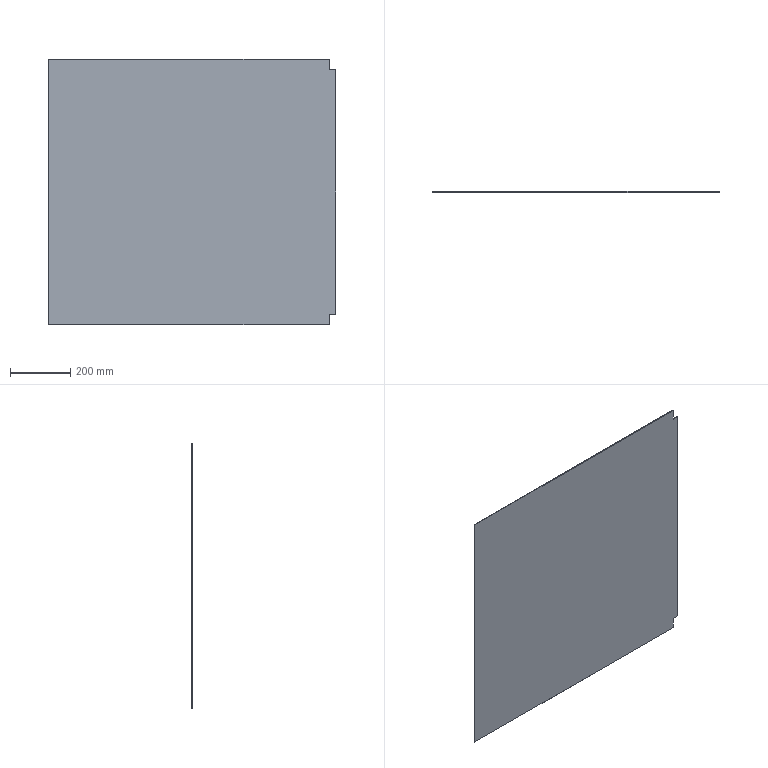Part | SolidWorks | features Extrusion 1 | 1 solid | 10 faces | box 956 x 3 x 885 mm | volume 2533644 mm3 | plane 10
STEP:
#1=CARTESIAN_POINT('',(-21.,0.,-406.5));
#2=VERTEX_POINT('',#1);
#3=CARTESIAN_POINT('',(-21.,0.,-442.5));
#4=VERTEX_POINT('',#3);
#5=CARTESIAN_POINT('',(-21.,0.,-406.5));
#6=DIRECTION('',(0.,0.,-1.));
#7=VECTOR('',#6,1000.);
#8=LINE('',#5,#7);
#9=EDGE_CURVE('',#2,#4,#8,.T.);
#10=ORIENTED_EDGE('',*,*,#9,.T.);
#11=CARTESIAN_POINT('',(-21.,3.,-442.5));
#12=VERTEX_POINT('',#11);
#13=CARTESIAN_POINT('',(-21.,3.,-442.5));
#14=DIRECTION('',(0.,-1.,0.));
#15=VECTOR('',#14,1000.);
#16=LINE('',#13,#15);
#17=EDGE_CURVE('',#12,#4,#16,.T.);
#18=ORIENTED_EDGE('',*,*,#17,.F.);
#19=CARTESIAN_POINT('',(-21.,3.,-406.5));
#20=VERTEX_POINT('',#19);
#21=CARTESIAN_POINT('',(-21.,3.,-406.5));
#22=DIRECTION('',(0.,0.,-1.));
#23=VECTOR('',#22,1000.);
#24=LINE('',#21,#23);
#25=EDGE_CURVE('',#20,#12,#24,.T.);
#26=ORIENTED_EDGE('',*,*,#25,.F.);
#27=CARTESIAN_POINT('',(-21.,3.,-406.5));
#28=DIRECTION('',(0.,-1.,0.));
#29=VECTOR('',#28,1000.);
#30=LINE('',#27,#29);
#31=EDGE_CURVE('',#20,#2,#30,.T.);
#32=ORIENTED_EDGE('',*,*,#31,.T.);
#33=EDGE_LOOP('',(#10,#18,#26,#32));
#34=FACE_OUTER_BOUND('',#33,.T.);
#35=CARTESIAN_POINT('',(-21.,3.,-406.5));
#36=DIRECTION('',(-1.,0.,0.));
#37=DIRECTION('',(0.,0.,1.));
#38=AXIS2_PLACEMENT_3D('',#35,#36,#37);
#39=PLANE('',#38);
#40=ADVANCED_FACE('',(#34),#39,.F.);
#41=CARTESIAN_POINT('',(-956.,0.,-442.5));
#42=VERTEX_POINT('',#41);
#43=CARTESIAN_POINT('',(-956.,0.,-442.5));
#44=DIRECTION('',(-1.,0.,0.));
#45=VECTOR('',#44,1000.);
#46=LINE('',#43,#45);
#47=EDGE_CURVE('',#4,#42,#46,.T.);
#48=ORIENTED_EDGE('',*,*,#47,.T.);
#49=CARTESIAN_POINT('',(-956.,3.,-442.5));
#50=VERTEX_POINT('',#49);
#51=CARTESIAN_POINT('',(-956.,3.,-442.5));
#52=DIRECTION('',(0.,-1.,0.));
#53=VECTOR('',#52,1000.);
#54=LINE('',#51,#53);
#55=EDGE_CURVE('',#50,#42,#54,.T.);
#56=ORIENTED_EDGE('',*,*,#55,.F.);
#57=CARTESIAN_POINT('',(-956.,3.,-442.5));
#58=DIRECTION('',(-1.,0.,0.));
#59=VECTOR('',#58,1000.);
#60=LINE('',#57,#59);
#61=EDGE_CURVE('',#12,#50,#60,.T.);
#62=ORIENTED_EDGE('',*,*,#61,.F.);
#63=ORIENTED_EDGE('',*,*,#17,.T.);
#64=EDGE_LOOP('',(#48,#56,#62,#63));
#65=FACE_OUTER_BOUND('',#64,.T.);
#66=CARTESIAN_POINT('',(-956.,3.,-442.5));
#67=DIRECTION('',(0.,0.,1.));
#68=DIRECTION('',(1.,0.,0.));
#69=AXIS2_PLACEMENT_3D('',#66,#67,#68);
#70=PLANE('',#69);
#71=ADVANCED_FACE('',(#65),#70,.F.);
#72=CARTESIAN_POINT('',(-956.,0.,442.5));
#73=VERTEX_POINT('',#72);
#74=CARTESIAN_POINT('',(-956.,0.,442.5));
#75=DIRECTION('',(0.,0.,1.));
#76=VECTOR('',#75,1000.);
#77=LINE('',#74,#76);
#78=EDGE_CURVE('',#42,#73,#77,.T.);
#79=ORIENTED_EDGE('',*,*,#78,.T.);
#80=CARTESIAN_POINT('',(-956.,3.,442.5));
#81=VERTEX_POINT('',#80);
#82=CARTESIAN_POINT('',(-956.,3.,442.5));
#83=DIRECTION('',(0.,-1.,0.));
#84=VECTOR('',#83,1000.);
#85=LINE('',#82,#84);
#86=EDGE_CURVE('',#81,#73,#85,.T.);
#87=ORIENTED_EDGE('',*,*,#86,.F.);
#88=CARTESIAN_POINT('',(-956.,3.,442.5));
#89=DIRECTION('',(0.,0.,1.));
#90=VECTOR('',#89,1000.);
#91=LINE('',#88,#90);
#92=EDGE_CURVE('',#50,#81,#91,.T.);
#93=ORIENTED_EDGE('',*,*,#92,.F.);
#94=ORIENTED_EDGE('',*,*,#55,.T.);
#95=EDGE_LOOP('',(#79,#87,#93,#94));
#96=FACE_OUTER_BOUND('',#95,.T.);
#97=CARTESIAN_POINT('',(-956.,3.,442.5));
#98=DIRECTION('',(1.,0.,0.));
#99=DIRECTION('',(0.,0.,-1.));
#100=AXIS2_PLACEMENT_3D('',#97,#98,#99);
#101=PLANE('',#100);
#102=ADVANCED_FACE('',(#96),#101,.F.);
#103=CARTESIAN_POINT('',(-21.,0.,442.5));
#104=VERTEX_POINT('',#103);
#105=CARTESIAN_POINT('',(-956.,0.,442.5));
#106=DIRECTION('',(1.,0.,0.));
#107=VECTOR('',#106,1000.);
#108=LINE('',#105,#107);
#109=EDGE_CURVE('',#73,#104,#108,.T.);
#110=ORIENTED_EDGE('',*,*,#109,.T.);
#111=CARTESIAN_POINT('',(-21.,3.,442.5));
#112=VERTEX_POINT('',#111);
#113=CARTESIAN_POINT('',(-21.,3.,442.5));
#114=DIRECTION('',(0.,-1.,0.));
#115=VECTOR('',#114,1000.);
#116=LINE('',#113,#115);
#117=EDGE_CURVE('',#112,#104,#116,.T.);
#118=ORIENTED_EDGE('',*,*,#117,.F.);
#119=CARTESIAN_POINT('',(-956.,3.,442.5));
#120=DIRECTION('',(1.,0.,0.));
#121=VECTOR('',#120,1000.);
#122=LINE('',#119,#121);
#123=EDGE_CURVE('',#81,#112,#122,.T.);
#124=ORIENTED_EDGE('',*,*,#123,.F.);
#125=ORIENTED_EDGE('',*,*,#86,.T.);
#126=EDGE_LOOP('',(#110,#118,#124,#125));
#127=FACE_OUTER_BOUND('',#126,.T.);
#128=CARTESIAN_POINT('',(-956.,3.,442.5));
#129=DIRECTION('',(0.,0.,-1.));
#130=DIRECTION('',(-1.,0.,0.));
#131=AXIS2_PLACEMENT_3D('',#128,#129,#130);
#132=PLANE('',#131);
#133=ADVANCED_FACE('',(#127),#132,.F.);
#134=CARTESIAN_POINT('',(-21.,0.,406.5));
#135=VERTEX_POINT('',#134);
#136=CARTESIAN_POINT('',(-21.,0.,406.5));
#137=DIRECTION('',(0.,0.,-1.));
#138=VECTOR('',#137,1000.);
#139=LINE('',#136,#138);
#140=EDGE_CURVE('',#104,#135,#139,.T.);
#141=ORIENTED_EDGE('',*,*,#140,.T.);
#142=CARTESIAN_POINT('',(-21.,3.,406.5));
#143=VERTEX_POINT('',#142);
#144=CARTESIAN_POINT('',(-21.,3.,406.5));
#145=DIRECTION('',(0.,-1.,0.));
#146=VECTOR('',#145,1000.);
#147=LINE('',#144,#146);
#148=EDGE_CURVE('',#143,#135,#147,.T.);
#149=ORIENTED_EDGE('',*,*,#148,.F.);
#150=CARTESIAN_POINT('',(-21.,3.,406.5));
#151=DIRECTION('',(0.,0.,-1.));
#152=VECTOR('',#151,1000.);
#153=LINE('',#150,#152);
#154=EDGE_CURVE('',#112,#143,#153,.T.);
#155=ORIENTED_EDGE('',*,*,#154,.F.);
#156=ORIENTED_EDGE('',*,*,#117,.T.);
#157=EDGE_LOOP('',(#141,#149,#155,#156));
#158=FACE_OUTER_BOUND('',#157,.T.);
#159=CARTESIAN_POINT('',(-21.,3.,406.5));
#160=DIRECTION('',(-1.,0.,0.));
#161=DIRECTION('',(0.,0.,1.));
#162=AXIS2_PLACEMENT_3D('',#159,#160,#161);
#163=PLANE('',#162);
#164=ADVANCED_FACE('',(#158),#163,.F.);
#165=CARTESIAN_POINT('',(0.,0.,406.5));
#166=VERTEX_POINT('',#165);
#167=CARTESIAN_POINT('',(-21.,0.,406.5));
#168=DIRECTION('',(1.,0.,0.));
#169=VECTOR('',#168,1000.);
#170=LINE('',#167,#169);
#171=EDGE_CURVE('',#135,#166,#170,.T.);
#172=ORIENTED_EDGE('',*,*,#171,.T.);
#173=CARTESIAN_POINT('',(0.,3.,406.5));
#174=VERTEX_POINT('',#173);
#175=CARTESIAN_POINT('',(0.,3.,406.5));
#176=DIRECTION('',(0.,-1.,0.));
#177=VECTOR('',#176,1000.);
#178=LINE('',#175,#177);
#179=EDGE_CURVE('',#174,#166,#178,.T.);
#180=ORIENTED_EDGE('',*,*,#179,.F.);
#181=CARTESIAN_POINT('',(-21.,3.,406.5));
#182=DIRECTION('',(1.,0.,0.));
#183=VECTOR('',#182,1000.);
#184=LINE('',#181,#183);
#185=EDGE_CURVE('',#143,#174,#184,.T.);
#186=ORIENTED_EDGE('',*,*,#185,.F.);
#187=ORIENTED_EDGE('',*,*,#148,.T.);
#188=EDGE_LOOP('',(#172,#180,#186,#187));
#189=FACE_OUTER_BOUND('',#188,.T.);
#190=CARTESIAN_POINT('',(-21.,3.,406.5));
#191=DIRECTION('',(0.,0.,-1.));
#192=DIRECTION('',(-1.,0.,0.));
#193=AXIS2_PLACEMENT_3D('',#190,#191,#192);
#194=PLANE('',#193);
#195=ADVANCED_FACE('',(#189),#194,.F.);
#196=CARTESIAN_POINT('',(0.,0.,-406.5));
#197=VERTEX_POINT('',#196);
#198=CARTESIAN_POINT('',(0.,0.,-406.5));
#199=DIRECTION('',(0.,0.,-1.));
#200=VECTOR('',#199,1000.);
#201=LINE('',#198,#200);
#202=EDGE_CURVE('',#166,#197,#201,.T.);
#203=ORIENTED_EDGE('',*,*,#202,.T.);
#204=CARTESIAN_POINT('',(0.,3.,-406.5));
#205=VERTEX_POINT('',#204);
#206=CARTESIAN_POINT('',(0.,3.,-406.5));
#207=DIRECTION('',(0.,-1.,0.));
#208=VECTOR('',#207,1000.);
#209=LINE('',#206,#208);
#210=EDGE_CURVE('',#205,#197,#209,.T.);
#211=ORIENTED_EDGE('',*,*,#210,.F.);
#212=CARTESIAN_POINT('',(0.,3.,-406.5));
#213=DIRECTION('',(0.,0.,-1.));
#214=VECTOR('',#213,1000.);
#215=LINE('',#212,#214);
#216=EDGE_CURVE('',#174,#205,#215,.T.);
#217=ORIENTED_EDGE('',*,*,#216,.F.);
#218=ORIENTED_EDGE('',*,*,#179,.T.);
#219=EDGE_LOOP('',(#203,#211,#217,#218));
#220=FACE_OUTER_BOUND('',#219,.T.);
#221=CARTESIAN_POINT('',(0.,3.,-406.5));
#222=DIRECTION('',(-1.,0.,0.));
#223=DIRECTION('',(0.,0.,1.));
#224=AXIS2_PLACEMENT_3D('',#221,#222,#223);
#225=PLANE('',#224);
#226=ADVANCED_FACE('',(#220),#225,.F.);
#227=CARTESIAN_POINT('',(-21.,0.,-406.5));
#228=DIRECTION('',(-1.,0.,0.));
#229=VECTOR('',#228,1000.);
#230=LINE('',#227,#229);
#231=EDGE_CURVE('',#197,#2,#230,.T.);
#232=ORIENTED_EDGE('',*,*,#231,.T.);
#233=ORIENTED_EDGE('',*,*,#31,.F.);
#234=CARTESIAN_POINT('',(-21.,3.,-406.5));
#235=DIRECTION('',(-1.,0.,0.));
#236=VECTOR('',#235,1000.);
#237=LINE('',#234,#236);
#238=EDGE_CURVE('',#205,#20,#237,.T.);
#239=ORIENTED_EDGE('',*,*,#238,.F.);
#240=ORIENTED_EDGE('',*,*,#210,.T.);
#241=EDGE_LOOP('',(#232,#233,#239,#240));
#242=FACE_OUTER_BOUND('',#241,.T.);
#243=CARTESIAN_POINT('',(-21.,3.,-406.5));
#244=DIRECTION('',(0.,0.,1.));
#245=DIRECTION('',(1.,0.,0.));
#246=AXIS2_PLACEMENT_3D('',#243,#244,#245);
#247=PLANE('',#246);
#248=ADVANCED_FACE('',(#242),#247,.F.);
#249=ORIENTED_EDGE('',*,*,#25,.T.);
#250=ORIENTED_EDGE('',*,*,#61,.T.);
#251=ORIENTED_EDGE('',*,*,#92,.T.);
#252=ORIENTED_EDGE('',*,*,#123,.T.);
#253=ORIENTED_EDGE('',*,*,#154,.T.);
#254=ORIENTED_EDGE('',*,*,#185,.T.);
#255=ORIENTED_EDGE('',*,*,#216,.T.);
#256=ORIENTED_EDGE('',*,*,#238,.T.);
#257=EDGE_LOOP('',(#249,#250,#251,#252,#253,#254,#255,#256));
#258=FACE_OUTER_BOUND('',#257,.T.);
#259=CARTESIAN_POINT('',(0.,3.,0.));
#260=DIRECTION('',(0.,-1.,0.));
#261=DIRECTION('',(0.,0.,-1.));
#262=AXIS2_PLACEMENT_3D('',#259,#260,#261);
#263=PLANE('',#262);
#264=ADVANCED_FACE('',(#258),#263,.F.);
#265=ORIENTED_EDGE('',*,*,#9,.F.);
#266=ORIENTED_EDGE('',*,*,#231,.F.);
#267=ORIENTED_EDGE('',*,*,#202,.F.);
#268=ORIENTED_EDGE('',*,*,#171,.F.);
#269=ORIENTED_EDGE('',*,*,#140,.F.);
#270=ORIENTED_EDGE('',*,*,#109,.F.);
#271=ORIENTED_EDGE('',*,*,#78,.F.);
#272=ORIENTED_EDGE('',*,*,#47,.F.);
#273=EDGE_LOOP('',(#265,#266,#267,#268,#269,#270,#271,#272));
#274=FACE_OUTER_BOUND('',#273,.T.);
#275=CARTESIAN_POINT('',(0.,0.,0.));
#276=DIRECTION('',(0.,-1.,0.));
#277=DIRECTION('',(0.,0.,-1.));
#278=AXIS2_PLACEMENT_3D('',#275,#276,#277);
#279=PLANE('',#278);
#280=ADVANCED_FACE('',(#274),#279,.T.);
#281=CLOSED_SHELL('',(#40,#71,#102,#133,#164,#195,#226,#248,#264,#280));
#282=MANIFOLD_SOLID_BREP('',#281);
#283=CARTESIAN_POINT('',(0.,0.,0.));
#284=DIRECTION('',(0.,0.,1.));
#285=DIRECTION('',(1.,0.,0.));
#286=AXIS2_PLACEMENT_3D('',#283,#284,#285);
#287=(LENGTH_UNIT()NAMED_UNIT(*)SI_UNIT(.MILLI.,.METRE.));
#288=UNCERTAINTY_MEASURE_WITH_UNIT(LENGTH_MEASURE(0.00001),#287,'','');
#289=(NAMED_UNIT(*)PLANE_ANGLE_UNIT()SI_UNIT($,.RADIAN.));
#290=(NAMED_UNIT(*)SI_UNIT($,.STERADIAN.)SOLID_ANGLE_UNIT());
#291=(GEOMETRIC_REPRESENTATION_CONTEXT(3)GLOBAL_UNCERTAINTY_ASSIGNED_CONTEXT((#288))GLOBAL_UNIT_ASSIGNED_CONTEXT((#287,#289,#290))REPRESENTATION_CONTEXT('',''));
#292=ADVANCED_BREP_SHAPE_REPRESENTATION('',(#282,#286),#291);